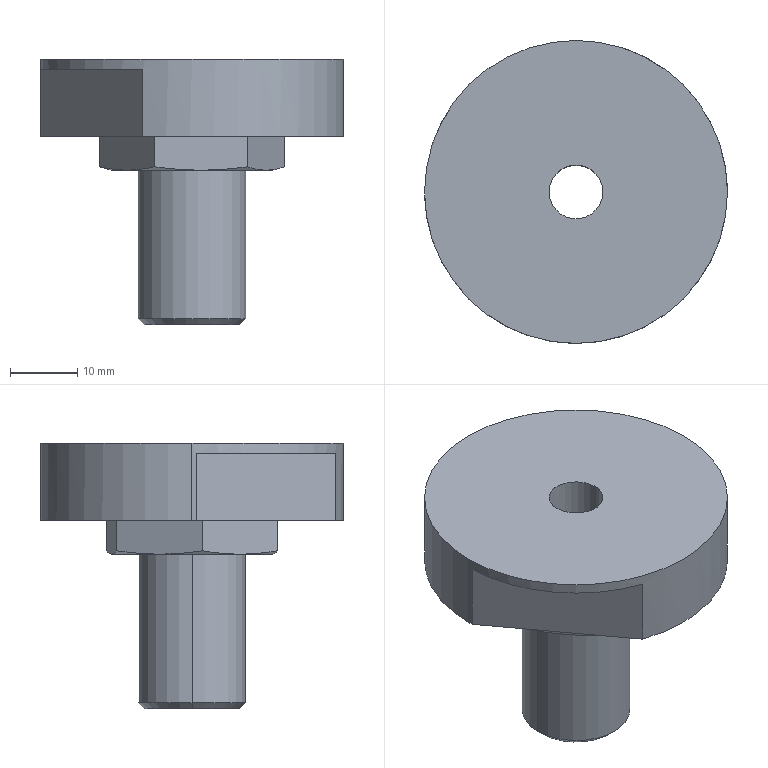Part | SolidWorks | features BaseBody 1 | 1 solid | 34 faces | box 45 x 45 x 39.5 mm | volume 21967 mm3 | plane 14 | cone 12 | cylinder 8 | commonest cylinder face diameters 8 x2 8.566 x2 16 x2 45 x2
STEP:
#1=CARTESIAN_POINT('',(67.28,21.29,385.481));
#2=VERTEX_POINT('',#1);
#3=CARTESIAN_POINT('',(37.5,0.,385.481));
#4=VERTEX_POINT('',#3);
#5=CARTESIAN_POINT('',(60.,0.,385.481));
#6=DIRECTION('',(0.,0.,1.));
#7=DIRECTION('',(1.,0.,0.));
#8=AXIS2_PLACEMENT_3D('',#5,#6,#7);
#9=CIRCLE('',#8,22.5);
#10=EDGE_CURVE('',#2,#4,#9,.T.);
#11=ORIENTED_EDGE('',*,*,#10,.T.);
#12=CARTESIAN_POINT('',(37.5,0.,396.981));
#13=VERTEX_POINT('',#12);
#14=CARTESIAN_POINT('',(37.5,0.,391.231));
#15=DIRECTION('',(0.,0.,1.));
#16=VECTOR('',#15,1000.);
#17=LINE('',#14,#16);
#18=EDGE_CURVE('',#4,#13,#17,.T.);
#19=ORIENTED_EDGE('',*,*,#18,.T.);
#20=CARTESIAN_POINT('',(82.5,0.,396.981));
#21=VERTEX_POINT('',#20);
#22=CARTESIAN_POINT('',(60.,0.,396.981));
#23=DIRECTION('',(0.,0.,1.));
#24=DIRECTION('',(1.,0.,0.));
#25=AXIS2_PLACEMENT_3D('',#22,#23,#24);
#26=CIRCLE('',#25,22.5);
#27=EDGE_CURVE('',#21,#13,#26,.T.);
#28=ORIENTED_EDGE('',*,*,#27,.F.);
#29=CARTESIAN_POINT('',(82.5,0.,385.481));
#30=VERTEX_POINT('',#29);
#31=CARTESIAN_POINT('',(82.5,0.,391.231));
#32=DIRECTION('',(0.,0.,1.));
#33=VECTOR('',#32,1000.);
#34=LINE('',#31,#33);
#35=EDGE_CURVE('',#30,#21,#34,.T.);
#36=ORIENTED_EDGE('',*,*,#35,.F.);
#37=CARTESIAN_POINT('',(82.49,0.6822,385.481));
#38=VERTEX_POINT('',#37);
#39=CARTESIAN_POINT('',(60.,0.,385.481));
#40=DIRECTION('',(0.,0.,1.));
#41=DIRECTION('',(1.,0.,0.));
#42=AXIS2_PLACEMENT_3D('',#39,#40,#41);
#43=CIRCLE('',#42,22.5);
#44=EDGE_CURVE('',#30,#38,#43,.T.);
#45=ORIENTED_EDGE('',*,*,#44,.T.);
#46=CARTESIAN_POINT('',(82.49,0.6822,395.481));
#47=VERTEX_POINT('',#46);
#48=CARTESIAN_POINT('',(82.49,0.6822,391.231));
#49=DIRECTION('',(0.,0.,1.));
#50=VECTOR('',#49,1000.);
#51=LINE('',#48,#50);
#52=EDGE_CURVE('',#38,#47,#51,.T.);
#53=ORIENTED_EDGE('',*,*,#52,.T.);
#54=CARTESIAN_POINT('',(67.28,21.29,395.481));
#55=VERTEX_POINT('',#54);
#56=CARTESIAN_POINT('',(60.,0.,395.481));
#57=DIRECTION('',(0.,0.,1.));
#58=DIRECTION('',(1.,0.,0.));
#59=AXIS2_PLACEMENT_3D('',#56,#57,#58);
#60=CIRCLE('',#59,22.5);
#61=EDGE_CURVE('',#47,#55,#60,.T.);
#62=ORIENTED_EDGE('',*,*,#61,.T.);
#63=CARTESIAN_POINT('',(67.28,21.29,391.231));
#64=DIRECTION('',(0.,0.,-1.));
#65=VECTOR('',#64,1000.);
#66=LINE('',#63,#65);
#67=EDGE_CURVE('',#55,#2,#66,.T.);
#68=ORIENTED_EDGE('',*,*,#67,.T.);
#69=EDGE_LOOP('',(#11,#19,#28,#36,#45,#53,#62,#68));
#70=FACE_OUTER_BOUND('',#69,.T.);
#71=CARTESIAN_POINT('',(60.,0.,391.231));
#72=DIRECTION('',(0.,0.,1.));
#73=DIRECTION('',(1.,0.,0.));
#74=AXIS2_PLACEMENT_3D('',#71,#72,#73);
#75=CYLINDRICAL_SURFACE('',#74,22.5);
#76=ADVANCED_FACE('',(#70),#75,.T.);
#77=CARTESIAN_POINT('',(56.,0.,361.844));
#78=VERTEX_POINT('',#77);
#79=CARTESIAN_POINT('',(64.,0.,361.844));
#80=VERTEX_POINT('',#79);
#81=CARTESIAN_POINT('',(60.,0.,361.844));
#82=DIRECTION('',(0.,0.,1.));
#83=DIRECTION('',(1.,0.,0.));
#84=AXIS2_PLACEMENT_3D('',#81,#82,#83);
#85=CIRCLE('',#84,4.);
#86=EDGE_CURVE('',#78,#80,#85,.T.);
#87=ORIENTED_EDGE('',*,*,#86,.F.);
#88=CARTESIAN_POINT('',(56.,0.,396.981));
#89=VERTEX_POINT('',#88);
#90=CARTESIAN_POINT('',(56.,0.,379.413));
#91=DIRECTION('',(0.,0.,1.));
#92=VECTOR('',#91,1000.);
#93=LINE('',#90,#92);
#94=EDGE_CURVE('',#78,#89,#93,.T.);
#95=ORIENTED_EDGE('',*,*,#94,.T.);
#96=CARTESIAN_POINT('',(64.,0.,396.981));
#97=VERTEX_POINT('',#96);
#98=CARTESIAN_POINT('',(60.,0.,396.981));
#99=DIRECTION('',(0.,0.,-1.));
#100=DIRECTION('',(1.,0.,0.));
#101=AXIS2_PLACEMENT_3D('',#98,#99,#100);
#102=CIRCLE('',#101,4.);
#103=EDGE_CURVE('',#97,#89,#102,.T.);
#104=ORIENTED_EDGE('',*,*,#103,.F.);
#105=CARTESIAN_POINT('',(64.,0.,379.413));
#106=DIRECTION('',(0.,0.,1.));
#107=VECTOR('',#106,1000.);
#108=LINE('',#105,#107);
#109=EDGE_CURVE('',#80,#97,#108,.T.);
#110=ORIENTED_EDGE('',*,*,#109,.F.);
#111=EDGE_LOOP('',(#87,#95,#104,#110));
#112=FACE_OUTER_BOUND('',#111,.T.);
#113=CARTESIAN_POINT('',(60.,0.,379.413));
#114=DIRECTION('',(0.,0.,1.));
#115=DIRECTION('',(1.,0.,0.));
#116=AXIS2_PLACEMENT_3D('',#113,#114,#115);
#117=CYLINDRICAL_SURFACE('',#116,4.);
#118=ADVANCED_FACE('',(#112),#117,.F.);
#119=ORIENTED_EDGE('',*,*,#86,.T.);
#120=CARTESIAN_POINT('',(64.283,0.,361.681));
#121=VERTEX_POINT('',#120);
#122=CARTESIAN_POINT('',(64.283,0.,361.681));
#123=DIRECTION('',(0.866,0.,-0.5));
#124=VECTOR('',#123,1000.);
#125=LINE('',#122,#124);
#126=EDGE_CURVE('',#80,#121,#125,.T.);
#127=ORIENTED_EDGE('',*,*,#126,.T.);
#128=CARTESIAN_POINT('',(55.717,0.,361.681));
#129=VERTEX_POINT('',#128);
#130=CARTESIAN_POINT('',(60.,0.,361.681));
#131=DIRECTION('',(0.,0.,1.));
#132=DIRECTION('',(-0.8046,-0.5938,0.));
#133=AXIS2_PLACEMENT_3D('',#130,#131,#132);
#134=CIRCLE('',#133,4.283);
#135=EDGE_CURVE('',#129,#121,#134,.T.);
#136=ORIENTED_EDGE('',*,*,#135,.F.);
#137=CARTESIAN_POINT('',(55.717,0.,361.681));
#138=DIRECTION('',(-0.866,0.,-0.5));
#139=VECTOR('',#138,1000.);
#140=LINE('',#137,#139);
#141=EDGE_CURVE('',#78,#129,#140,.T.);
#142=ORIENTED_EDGE('',*,*,#141,.F.);
#143=EDGE_LOOP('',(#119,#127,#136,#142));
#144=FACE_OUTER_BOUND('',#143,.T.);
#145=CARTESIAN_POINT('',(60.,0.,361.681));
#146=DIRECTION('',(0.,0.,-1.));
#147=DIRECTION('',(-1.,0.,0.));
#148=AXIS2_PLACEMENT_3D('',#145,#146,#147);
#149=CONICAL_SURFACE('',#148,4.283,1.047);
#150=ADVANCED_FACE('',(#144),#149,.F.);
#151=CARTESIAN_POINT('',(55.717,0.,358.062));
#152=VERTEX_POINT('',#151);
#153=CARTESIAN_POINT('',(64.283,0.,358.062));
#154=VERTEX_POINT('',#153);
#155=CARTESIAN_POINT('',(60.,0.,358.062));
#156=DIRECTION('',(0.,0.,1.));
#157=DIRECTION('',(1.,0.,0.));
#158=AXIS2_PLACEMENT_3D('',#155,#156,#157);
#159=CIRCLE('',#158,4.283);
#160=EDGE_CURVE('',#152,#154,#159,.T.);
#161=ORIENTED_EDGE('',*,*,#160,.F.);
#162=CARTESIAN_POINT('',(55.717,0.,358.872));
#163=DIRECTION('',(0.,0.,1.));
#164=VECTOR('',#163,1000.);
#165=LINE('',#162,#164);
#166=EDGE_CURVE('',#152,#129,#165,.T.);
#167=ORIENTED_EDGE('',*,*,#166,.T.);
#168=ORIENTED_EDGE('',*,*,#135,.T.);
#169=CARTESIAN_POINT('',(64.283,0.,358.872));
#170=DIRECTION('',(0.,0.,1.));
#171=VECTOR('',#170,1000.);
#172=LINE('',#169,#171);
#173=EDGE_CURVE('',#154,#121,#172,.T.);
#174=ORIENTED_EDGE('',*,*,#173,.F.);
#175=EDGE_LOOP('',(#161,#167,#168,#174));
#176=FACE_OUTER_BOUND('',#175,.T.);
#177=CARTESIAN_POINT('',(60.,0.,358.872));
#178=DIRECTION('',(0.,0.,1.));
#179=DIRECTION('',(1.,0.,0.));
#180=AXIS2_PLACEMENT_3D('',#177,#178,#179);
#181=CYLINDRICAL_SURFACE('',#180,4.283);
#182=ADVANCED_FACE('',(#176),#181,.F.);
#183=ORIENTED_EDGE('',*,*,#160,.T.);
#184=CARTESIAN_POINT('',(64.864,0.,357.481));
#185=VERTEX_POINT('',#184);
#186=CARTESIAN_POINT('',(64.864,0.,357.481));
#187=DIRECTION('',(0.7071,0.,-0.7071));
#188=VECTOR('',#187,1000.);
#189=LINE('',#186,#188);
#190=EDGE_CURVE('',#154,#185,#189,.T.);
#191=ORIENTED_EDGE('',*,*,#190,.T.);
#192=CARTESIAN_POINT('',(55.136,0.,357.481));
#193=VERTEX_POINT('',#192);
#194=CARTESIAN_POINT('',(60.,0.,357.481));
#195=DIRECTION('',(0.,0.,1.));
#196=DIRECTION('',(-1.,0.,0.));
#197=AXIS2_PLACEMENT_3D('',#194,#195,#196);
#198=CIRCLE('',#197,4.864);
#199=EDGE_CURVE('',#193,#185,#198,.T.);
#200=ORIENTED_EDGE('',*,*,#199,.F.);
#201=CARTESIAN_POINT('',(55.136,0.,357.481));
#202=DIRECTION('',(-0.7071,0.,-0.7071));
#203=VECTOR('',#202,1000.);
#204=LINE('',#201,#203);
#205=EDGE_CURVE('',#152,#193,#204,.T.);
#206=ORIENTED_EDGE('',*,*,#205,.F.);
#207=EDGE_LOOP('',(#183,#191,#200,#206));
#208=FACE_OUTER_BOUND('',#207,.T.);
#209=CARTESIAN_POINT('',(60.,0.,357.481));
#210=DIRECTION('',(0.,0.,-1.));
#211=DIRECTION('',(-1.,0.,0.));
#212=AXIS2_PLACEMENT_3D('',#209,#210,#211);
#213=CONICAL_SURFACE('',#212,4.864,0.7854);
#214=ADVANCED_FACE('',(#208),#213,.F.);
#215=CARTESIAN_POINT('',(68.,0.,358.401));
#216=VERTEX_POINT('',#215);
#217=CARTESIAN_POINT('',(52.,0.,358.401));
#218=VERTEX_POINT('',#217);
#219=CARTESIAN_POINT('',(60.,0.,358.401));
#220=DIRECTION('',(0.,0.,1.));
#221=DIRECTION('',(1.,0.,0.));
#222=AXIS2_PLACEMENT_3D('',#219,#220,#221);
#223=CIRCLE('',#222,8.);
#224=EDGE_CURVE('',#216,#218,#223,.T.);
#225=ORIENTED_EDGE('',*,*,#224,.T.);
#226=CARTESIAN_POINT('',(52.,0.,380.481));
#227=VERTEX_POINT('',#226);
#228=CARTESIAN_POINT('',(52.,0.,368.441));
#229=DIRECTION('',(0.,0.,1.));
#230=VECTOR('',#229,1000.);
#231=LINE('',#228,#230);
#232=EDGE_CURVE('',#218,#227,#231,.T.);
#233=ORIENTED_EDGE('',*,*,#232,.T.);
#234=CARTESIAN_POINT('',(68.,0.,380.481));
#235=VERTEX_POINT('',#234);
#236=CARTESIAN_POINT('',(60.,0.,380.481));
#237=DIRECTION('',(0.,0.,1.));
#238=DIRECTION('',(1.,0.,0.));
#239=AXIS2_PLACEMENT_3D('',#236,#237,#238);
#240=CIRCLE('',#239,8.);
#241=EDGE_CURVE('',#235,#227,#240,.T.);
#242=ORIENTED_EDGE('',*,*,#241,.F.);
#243=CARTESIAN_POINT('',(68.,0.,368.441));
#244=DIRECTION('',(0.,0.,1.));
#245=VECTOR('',#244,1000.);
#246=LINE('',#243,#245);
#247=EDGE_CURVE('',#216,#235,#246,.T.);
#248=ORIENTED_EDGE('',*,*,#247,.F.);
#249=EDGE_LOOP('',(#225,#233,#242,#248));
#250=FACE_OUTER_BOUND('',#249,.T.);
#251=CARTESIAN_POINT('',(60.,0.,368.441));
#252=DIRECTION('',(0.,0.,1.));
#253=DIRECTION('',(1.,0.,0.));
#254=AXIS2_PLACEMENT_3D('',#251,#252,#253);
#255=CYLINDRICAL_SURFACE('',#254,8.);
#256=ADVANCED_FACE('',(#250),#255,.T.);
#257=CARTESIAN_POINT('',(52.92,0.,357.481));
#258=VERTEX_POINT('',#257);
#259=CARTESIAN_POINT('',(67.08,0.,357.481));
#260=VERTEX_POINT('',#259);
#261=CARTESIAN_POINT('',(60.,0.,357.481));
#262=DIRECTION('',(0.,0.,-1.));
#263=DIRECTION('',(1.,0.,0.));
#264=AXIS2_PLACEMENT_3D('',#261,#262,#263);
#265=CIRCLE('',#264,7.08);
#266=EDGE_CURVE('',#258,#260,#265,.T.);
#267=ORIENTED_EDGE('',*,*,#266,.F.);
#268=CARTESIAN_POINT('',(52.,0.,358.401));
#269=DIRECTION('',(-0.7071,0.,0.7071));
#270=VECTOR('',#269,1000.);
#271=LINE('',#268,#270);
#272=EDGE_CURVE('',#258,#218,#271,.T.);
#273=ORIENTED_EDGE('',*,*,#272,.T.);
#274=ORIENTED_EDGE('',*,*,#224,.F.);
#275=CARTESIAN_POINT('',(68.,0.,358.401));
#276=DIRECTION('',(0.7071,0.,0.7071));
#277=VECTOR('',#276,1000.);
#278=LINE('',#275,#277);
#279=EDGE_CURVE('',#260,#216,#278,.T.);
#280=ORIENTED_EDGE('',*,*,#279,.F.);
#281=EDGE_LOOP('',(#267,#273,#274,#280));
#282=FACE_OUTER_BOUND('',#281,.T.);
#283=CARTESIAN_POINT('',(60.,0.,358.401));
#284=DIRECTION('',(0.,0.,1.));
#285=DIRECTION('',(1.,0.,0.));
#286=AXIS2_PLACEMENT_3D('',#283,#284,#285);
#287=CONICAL_SURFACE('',#286,8.,0.7854);
#288=ADVANCED_FACE('',(#282),#287,.T.);
#289=ORIENTED_EDGE('',*,*,#27,.T.);
#290=CARTESIAN_POINT('',(60.,0.,396.981));
#291=DIRECTION('',(0.,0.,1.));
#292=DIRECTION('',(1.,0.,0.));
#293=AXIS2_PLACEMENT_3D('',#290,#291,#292);
#294=CIRCLE('',#293,22.5);
#295=EDGE_CURVE('',#13,#21,#294,.T.);
#296=ORIENTED_EDGE('',*,*,#295,.T.);
#297=EDGE_LOOP('',(#289,#296));
#298=FACE_OUTER_BOUND('',#297,.T.);
#299=ORIENTED_EDGE('',*,*,#103,.T.);
#300=CARTESIAN_POINT('',(60.,0.,396.981));
#301=DIRECTION('',(0.,0.,-1.));
#302=DIRECTION('',(1.,0.,0.));
#303=AXIS2_PLACEMENT_3D('',#300,#301,#302);
#304=CIRCLE('',#303,4.);
#305=EDGE_CURVE('',#89,#97,#304,.T.);
#306=ORIENTED_EDGE('',*,*,#305,.T.);
#307=EDGE_LOOP('',(#299,#306));
#308=FACE_BOUND('',#307,.T.);
#309=CARTESIAN_POINT('',(52.132,10.661,396.981));
#310=DIRECTION('',(0.,0.,1.));
#311=DIRECTION('',(1.,0.,0.));
#312=AXIS2_PLACEMENT_3D('',#309,#310,#311);
#313=PLANE('',#312);
#314=ADVANCED_FACE('',(#298,#308),#313,.T.);
#315=ORIENTED_EDGE('',*,*,#18,.F.);
#316=CARTESIAN_POINT('',(37.51,-0.6822,385.481));
#317=VERTEX_POINT('',#316);
#318=CARTESIAN_POINT('',(60.,0.,385.481));
#319=DIRECTION('',(0.,0.,1.));
#320=DIRECTION('',(1.,0.,0.));
#321=AXIS2_PLACEMENT_3D('',#318,#319,#320);
#322=CIRCLE('',#321,22.5);
#323=EDGE_CURVE('',#4,#317,#322,.T.);
#324=ORIENTED_EDGE('',*,*,#323,.T.);
#325=CARTESIAN_POINT('',(37.51,-0.6822,395.481));
#326=VERTEX_POINT('',#325);
#327=CARTESIAN_POINT('',(37.51,-0.6822,391.231));
#328=DIRECTION('',(0.,0.,1.));
#329=VECTOR('',#328,1000.);
#330=LINE('',#327,#329);
#331=EDGE_CURVE('',#317,#326,#330,.T.);
#332=ORIENTED_EDGE('',*,*,#331,.T.);
#333=CARTESIAN_POINT('',(52.72,-21.29,395.481));
#334=VERTEX_POINT('',#333);
#335=CARTESIAN_POINT('',(60.,0.,395.481));
#336=DIRECTION('',(0.,0.,1.));
#337=DIRECTION('',(1.,0.,0.));
#338=AXIS2_PLACEMENT_3D('',#335,#336,#337);
#339=CIRCLE('',#338,22.5);
#340=EDGE_CURVE('',#326,#334,#339,.T.);
#341=ORIENTED_EDGE('',*,*,#340,.T.);
#342=CARTESIAN_POINT('',(52.72,-21.29,385.481));
#343=VERTEX_POINT('',#342);
#344=CARTESIAN_POINT('',(52.72,-21.29,391.231));
#345=DIRECTION('',(0.,0.,-1.));
#346=VECTOR('',#345,1000.);
#347=LINE('',#344,#346);
#348=EDGE_CURVE('',#334,#343,#347,.T.);
#349=ORIENTED_EDGE('',*,*,#348,.T.);
#350=CARTESIAN_POINT('',(60.,0.,385.481));
#351=DIRECTION('',(0.,0.,1.));
#352=DIRECTION('',(1.,0.,0.));
#353=AXIS2_PLACEMENT_3D('',#350,#351,#352);
#354=CIRCLE('',#353,22.5);
#355=EDGE_CURVE('',#343,#30,#354,.T.);
#356=ORIENTED_EDGE('',*,*,#355,.T.);
#357=ORIENTED_EDGE('',*,*,#35,.T.);
#358=ORIENTED_EDGE('',*,*,#295,.F.);
#359=EDGE_LOOP('',(#315,#324,#332,#341,#349,#356,#357,#358));
#360=FACE_OUTER_BOUND('',#359,.T.);
#361=CARTESIAN_POINT('',(60.,0.,391.231));
#362=DIRECTION('',(0.,0.,1.));
#363=DIRECTION('',(1.,0.,0.));
#364=AXIS2_PLACEMENT_3D('',#361,#362,#363);
#365=CYLINDRICAL_SURFACE('',#364,22.5);
#366=ADVANCED_FACE('',(#360),#365,.T.);
#367=ORIENTED_EDGE('',*,*,#94,.F.);
#368=CARTESIAN_POINT('',(60.,0.,361.844));
#369=DIRECTION('',(0.,0.,1.));
#370=DIRECTION('',(1.,0.,0.));
#371=AXIS2_PLACEMENT_3D('',#368,#369,#370);
#372=CIRCLE('',#371,4.);
#373=EDGE_CURVE('',#80,#78,#372,.T.);
#374=ORIENTED_EDGE('',*,*,#373,.F.);
#375=ORIENTED_EDGE('',*,*,#109,.T.);
#376=ORIENTED_EDGE('',*,*,#305,.F.);
#377=EDGE_LOOP('',(#367,#374,#375,#376));
#378=FACE_OUTER_BOUND('',#377,.T.);
#379=CARTESIAN_POINT('',(60.,0.,379.413));
#380=DIRECTION('',(0.,0.,1.));
#381=DIRECTION('',(1.,0.,0.));
#382=AXIS2_PLACEMENT_3D('',#379,#380,#381);
#383=CYLINDRICAL_SURFACE('',#382,4.);
#384=ADVANCED_FACE('',(#378),#383,.F.);
#385=CARTESIAN_POINT('',(52.72,-21.29,385.481));
#386=DIRECTION('',(-0.5938,0.8046,0.));
#387=VECTOR('',#386,1000.);
#388=LINE('',#385,#387);
#389=EDGE_CURVE('',#343,#317,#388,.T.);
#390=ORIENTED_EDGE('',*,*,#389,.T.);
#391=ORIENTED_EDGE('',*,*,#323,.F.);
#392=ORIENTED_EDGE('',*,*,#10,.F.);
#393=CARTESIAN_POINT('',(67.28,21.29,385.481));
#394=DIRECTION('',(0.5938,-0.8046,0.));
#395=VECTOR('',#394,1000.);
#396=LINE('',#393,#395);
#397=EDGE_CURVE('',#2,#38,#396,.T.);
#398=ORIENTED_EDGE('',*,*,#397,.T.);
#399=ORIENTED_EDGE('',*,*,#44,.F.);
#400=ORIENTED_EDGE('',*,*,#355,.F.);
#401=EDGE_LOOP('',(#390,#391,#392,#398,#399,#400));
#402=FACE_OUTER_BOUND('',#401,.T.);
#403=CARTESIAN_POINT('',(65.541,12.7,385.481));
#404=VERTEX_POINT('',#403);
#405=CARTESIAN_POINT('',(51.772,11.149,385.481));
#406=VERTEX_POINT('',#405);
#407=CARTESIAN_POINT('',(65.541,12.7,385.481));
#408=DIRECTION('',(-0.9937,-0.112,0.));
#409=VECTOR('',#408,1000.);
#410=LINE('',#407,#409);
#411=EDGE_CURVE('',#404,#406,#410,.T.);
#412=ORIENTED_EDGE('',*,*,#411,.T.);
#413=CARTESIAN_POINT('',(46.231,-1.552,385.481));
#414=VERTEX_POINT('',#413);
#415=CARTESIAN_POINT('',(51.772,11.149,385.481));
#416=DIRECTION('',(-0.3999,-0.9166,0.));
#417=VECTOR('',#416,1000.);
#418=LINE('',#415,#417);
#419=EDGE_CURVE('',#406,#414,#418,.T.);
#420=ORIENTED_EDGE('',*,*,#419,.T.);
#421=CARTESIAN_POINT('',(54.459,-12.7,385.481));
#422=VERTEX_POINT('',#421);
#423=CARTESIAN_POINT('',(46.231,-1.552,385.481));
#424=DIRECTION('',(0.5938,-0.8046,0.));
#425=VECTOR('',#424,1000.);
#426=LINE('',#423,#425);
#427=EDGE_CURVE('',#414,#422,#426,.T.);
#428=ORIENTED_EDGE('',*,*,#427,.T.);
#429=CARTESIAN_POINT('',(68.228,-11.149,385.481));
#430=VERTEX_POINT('',#429);
#431=CARTESIAN_POINT('',(54.459,-12.7,385.481));
#432=DIRECTION('',(0.9937,0.112,0.));
#433=VECTOR('',#432,1000.);
#434=LINE('',#431,#433);
#435=EDGE_CURVE('',#422,#430,#434,.T.);
#436=ORIENTED_EDGE('',*,*,#435,.T.);
#437=CARTESIAN_POINT('',(73.769,1.552,385.481));
#438=VERTEX_POINT('',#437);
#439=CARTESIAN_POINT('',(68.228,-11.149,385.481));
#440=DIRECTION('',(0.3999,0.9166,0.));
#441=VECTOR('',#440,1000.);
#442=LINE('',#439,#441);
#443=EDGE_CURVE('',#430,#438,#442,.T.);
#444=ORIENTED_EDGE('',*,*,#443,.T.);
#445=CARTESIAN_POINT('',(73.769,1.552,385.481));
#446=DIRECTION('',(-0.5938,0.8046,0.));
#447=VECTOR('',#446,1000.);
#448=LINE('',#445,#447);
#449=EDGE_CURVE('',#438,#404,#448,.T.);
#450=ORIENTED_EDGE('',*,*,#449,.T.);
#451=EDGE_LOOP('',(#412,#420,#428,#436,#444,#450));
#452=FACE_BOUND('',#451,.T.);
#453=CARTESIAN_POINT('',(47.619,16.776,385.481));
#454=DIRECTION('',(0.,0.,-1.));
#455=DIRECTION('',(-1.,0.,0.));
#456=AXIS2_PLACEMENT_3D('',#453,#454,#455);
#457=PLANE('',#456);
#458=ADVANCED_FACE('',(#402,#452),#457,.T.);
#459=ORIENTED_EDGE('',*,*,#67,.F.);
#460=CARTESIAN_POINT('',(51.131,43.169,395.481));
#461=DIRECTION('',(-0.5938,0.8046,0.));
#462=VECTOR('',#461,1000.);
#463=LINE('',#460,#462);
#464=EDGE_CURVE('',#47,#55,#463,.T.);
#465=ORIENTED_EDGE('',*,*,#464,.F.);
#466=ORIENTED_EDGE('',*,*,#52,.F.);
#467=ORIENTED_EDGE('',*,*,#397,.F.);
#468=EDGE_LOOP('',(#459,#465,#466,#467));
#469=FACE_OUTER_BOUND('',#468,.T.);
#470=CARTESIAN_POINT('',(51.131,43.169,395.481));
#471=DIRECTION('',(-0.8046,-0.5938,0.));
#472=DIRECTION('',(0.5938,-0.8046,0.));
#473=AXIS2_PLACEMENT_3D('',#470,#471,#472);
#474=PLANE('',#473);
#475=ADVANCED_FACE('',(#469),#474,.F.);
#476=ORIENTED_EDGE('',*,*,#61,.F.);
#477=ORIENTED_EDGE('',*,*,#464,.T.);
#478=EDGE_LOOP('',(#476,#477));
#479=FACE_OUTER_BOUND('',#478,.T.);
#480=CARTESIAN_POINT('',(60.,0.,395.481));
#481=DIRECTION('',(0.,0.,-1.));
#482=DIRECTION('',(-1.,0.,0.));
#483=AXIS2_PLACEMENT_3D('',#480,#481,#482);
#484=PLANE('',#483);
#485=ADVANCED_FACE('',(#479),#484,.T.);
#486=ORIENTED_EDGE('',*,*,#348,.F.);
#487=CARTESIAN_POINT('',(68.869,-43.169,395.481));
#488=DIRECTION('',(0.5938,-0.8046,0.));
#489=VECTOR('',#488,1000.);
#490=LINE('',#487,#489);
#491=EDGE_CURVE('',#326,#334,#490,.T.);
#492=ORIENTED_EDGE('',*,*,#491,.F.);
#493=ORIENTED_EDGE('',*,*,#331,.F.);
#494=ORIENTED_EDGE('',*,*,#389,.F.);
#495=EDGE_LOOP('',(#486,#492,#493,#494));
#496=FACE_OUTER_BOUND('',#495,.T.);
#497=CARTESIAN_POINT('',(68.869,-43.169,395.481));
#498=DIRECTION('',(0.8046,0.5938,0.));
#499=DIRECTION('',(-0.5938,0.8046,0.));
#500=AXIS2_PLACEMENT_3D('',#497,#498,#499);
#501=PLANE('',#500);
#502=ADVANCED_FACE('',(#496),#501,.F.);
#503=ORIENTED_EDGE('',*,*,#340,.F.);
#504=ORIENTED_EDGE('',*,*,#491,.T.);
#505=EDGE_LOOP('',(#503,#504));
#506=FACE_OUTER_BOUND('',#505,.T.);
#507=CARTESIAN_POINT('',(60.,0.,395.481));
#508=DIRECTION('',(0.,0.,-1.));
#509=DIRECTION('',(-1.,0.,0.));
#510=AXIS2_PLACEMENT_3D('',#507,#508,#509);
#511=PLANE('',#510);
#512=ADVANCED_FACE('',(#506),#511,.T.);
#513=ORIENTED_EDGE('',*,*,#126,.F.);
#514=ORIENTED_EDGE('',*,*,#373,.T.);
#515=ORIENTED_EDGE('',*,*,#141,.T.);
#516=CARTESIAN_POINT('',(60.,0.,361.681));
#517=DIRECTION('',(0.,0.,1.));
#518=DIRECTION('',(-0.8046,-0.5938,0.));
#519=AXIS2_PLACEMENT_3D('',#516,#517,#518);
#520=CIRCLE('',#519,4.283);
#521=EDGE_CURVE('',#121,#129,#520,.T.);
#522=ORIENTED_EDGE('',*,*,#521,.F.);
#523=EDGE_LOOP('',(#513,#514,#515,#522));
#524=FACE_OUTER_BOUND('',#523,.T.);
#525=CARTESIAN_POINT('',(60.,0.,361.681));
#526=DIRECTION('',(0.,0.,-1.));
#527=DIRECTION('',(-1.,0.,0.));
#528=AXIS2_PLACEMENT_3D('',#525,#526,#527);
#529=CONICAL_SURFACE('',#528,4.283,1.047);
#530=ADVANCED_FACE('',(#524),#529,.F.);
#531=CARTESIAN_POINT('',(46.231,-1.552,380.978));
#532=VERTEX_POINT('',#531);
#533=CARTESIAN_POINT('',(46.231,-1.552,385.481));
#534=DIRECTION('',(0.,0.,-1.));
#535=VECTOR('',#534,1000.);
#536=LINE('',#533,#535);
#537=EDGE_CURVE('',#414,#532,#536,.T.);
#538=ORIENTED_EDGE('',*,*,#537,.F.);
#539=ORIENTED_EDGE('',*,*,#419,.F.);
#540=CARTESIAN_POINT('',(51.772,11.149,380.978));
#541=VERTEX_POINT('',#540);
#542=CARTESIAN_POINT('',(51.772,11.149,385.481));
#543=DIRECTION('',(0.,0.,1.));
#544=VECTOR('',#543,1000.);
#545=LINE('',#542,#544);
#546=EDGE_CURVE('',#541,#406,#545,.T.);
#547=ORIENTED_EDGE('',*,*,#546,.F.);
#548=CARTESIAN_POINT('',(49.001,4.798,380.481));
#549=VERTEX_POINT('',#548);
#550=CARTESIAN_POINT('',(49.001,4.798,380.481));
#551=CARTESIAN_POINT('',(49.465,5.862,380.481));
#552=CARTESIAN_POINT('',(49.928,6.923,380.527));
#553=CARTESIAN_POINT('',(50.851,9.039,380.699));
#554=CARTESIAN_POINT('',(51.312,10.095,380.824));
#555=CARTESIAN_POINT('',(51.772,11.149,380.978));
#556=B_SPLINE_CURVE_WITH_KNOTS('',3,(#550,#551,#552,#553,#554,#555),.UNSPECIFIED.,.F.,.F.,(4,2,4),(0.,0.003473,0.006946),.UNSPECIFIED.);
#557=EDGE_CURVE('',#549,#541,#556,.T.);
#558=ORIENTED_EDGE('',*,*,#557,.F.);
#559=CARTESIAN_POINT('',(46.231,-1.552,380.978));
#560=CARTESIAN_POINT('',(46.69,-0.498,380.824));
#561=CARTESIAN_POINT('',(47.151,0.5576,380.699));
#562=CARTESIAN_POINT('',(48.074,2.674,380.527));
#563=CARTESIAN_POINT('',(48.537,3.735,380.481));
#564=CARTESIAN_POINT('',(49.001,4.798,380.481));
#565=B_SPLINE_CURVE_WITH_KNOTS('',3,(#559,#560,#561,#562,#563,#564),.UNSPECIFIED.,.F.,.F.,(4,2,4),(0.,0.003473,0.006946),.UNSPECIFIED.);
#566=EDGE_CURVE('',#532,#549,#565,.T.);
#567=ORIENTED_EDGE('',*,*,#566,.F.);
#568=EDGE_LOOP('',(#538,#539,#547,#558,#567));
#569=FACE_OUTER_BOUND('',#568,.T.);
#570=CARTESIAN_POINT('',(46.231,-1.552,385.481));
#571=DIRECTION('',(0.9166,-0.3999,0.));
#572=DIRECTION('',(0.3999,0.9166,0.));
#573=AXIS2_PLACEMENT_3D('',#570,#571,#572);
#574=PLANE('',#573);
#575=ADVANCED_FACE('',(#569),#574,.F.);
#576=ORIENTED_EDGE('',*,*,#411,.F.);
#577=CARTESIAN_POINT('',(65.541,12.7,380.978));
#578=VERTEX_POINT('',#577);
#579=CARTESIAN_POINT('',(65.541,12.7,385.481));
#580=DIRECTION('',(0.,0.,1.));
#581=VECTOR('',#580,1000.);
#582=LINE('',#579,#581);
#583=EDGE_CURVE('',#578,#404,#582,.T.);
#584=ORIENTED_EDGE('',*,*,#583,.F.);
#585=CARTESIAN_POINT('',(58.656,11.925,380.481));
#586=VERTEX_POINT('',#585);
#587=CARTESIAN_POINT('',(58.656,11.925,380.481));
#588=CARTESIAN_POINT('',(59.81,12.054,380.481));
#589=CARTESIAN_POINT('',(60.96,12.184,380.527));
#590=CARTESIAN_POINT('',(63.254,12.443,380.699));
#591=CARTESIAN_POINT('',(64.398,12.572,380.824));
#592=CARTESIAN_POINT('',(65.541,12.7,380.978));
#593=B_SPLINE_CURVE_WITH_KNOTS('',3,(#587,#588,#589,#590,#591,#592),.UNSPECIFIED.,.F.,.F.,(4,2,4),(0.,0.003473,0.006946),.UNSPECIFIED.);
#594=EDGE_CURVE('',#586,#578,#593,.T.);
#595=ORIENTED_EDGE('',*,*,#594,.F.);
#596=CARTESIAN_POINT('',(51.772,11.149,380.978));
#597=CARTESIAN_POINT('',(52.914,11.277,380.824));
#598=CARTESIAN_POINT('',(54.058,11.406,380.699));
#599=CARTESIAN_POINT('',(56.353,11.665,380.527));
#600=CARTESIAN_POINT('',(57.503,11.795,380.481));
#601=CARTESIAN_POINT('',(58.656,11.925,380.481));
#602=B_SPLINE_CURVE_WITH_KNOTS('',3,(#596,#597,#598,#599,#600,#601),.UNSPECIFIED.,.F.,.F.,(4,2,4),(0.,0.003473,0.006946),.UNSPECIFIED.);
#603=EDGE_CURVE('',#541,#586,#602,.T.);
#604=ORIENTED_EDGE('',*,*,#603,.F.);
#605=ORIENTED_EDGE('',*,*,#546,.T.);
#606=EDGE_LOOP('',(#576,#584,#595,#604,#605));
#607=FACE_OUTER_BOUND('',#606,.T.);
#608=CARTESIAN_POINT('',(51.772,11.149,385.481));
#609=DIRECTION('',(0.112,-0.9937,0.));
#610=DIRECTION('',(0.9937,0.112,0.));
#611=AXIS2_PLACEMENT_3D('',#608,#609,#610);
#612=PLANE('',#611);
#613=ADVANCED_FACE('',(#607),#612,.F.);
#614=ORIENTED_EDGE('',*,*,#449,.F.);
#615=CARTESIAN_POINT('',(73.769,1.552,380.978));
#616=VERTEX_POINT('',#615);
#617=CARTESIAN_POINT('',(73.769,1.552,385.481));
#618=DIRECTION('',(0.,0.,1.));
#619=VECTOR('',#618,1000.);
#620=LINE('',#617,#619);
#621=EDGE_CURVE('',#616,#438,#620,.T.);
#622=ORIENTED_EDGE('',*,*,#621,.F.);
#623=CARTESIAN_POINT('',(69.655,7.126,380.481));
#624=VERTEX_POINT('',#623);
#625=CARTESIAN_POINT('',(69.655,7.126,380.481));
#626=CARTESIAN_POINT('',(70.344,6.192,380.481));
#627=CARTESIAN_POINT('',(71.032,5.261,380.527));
#628=CARTESIAN_POINT('',(72.403,3.403,380.699));
#629=CARTESIAN_POINT('',(73.087,2.477,380.824));
#630=CARTESIAN_POINT('',(73.769,1.552,380.978));
#631=B_SPLINE_CURVE_WITH_KNOTS('',3,(#625,#626,#627,#628,#629,#630),.UNSPECIFIED.,.F.,.F.,(4,2,4),(0.,0.003473,0.006946),.UNSPECIFIED.);
#632=EDGE_CURVE('',#624,#616,#631,.T.);
#633=ORIENTED_EDGE('',*,*,#632,.F.);
#634=CARTESIAN_POINT('',(65.541,12.7,380.978));
#635=CARTESIAN_POINT('',(66.223,11.775,380.824));
#636=CARTESIAN_POINT('',(66.907,10.849,380.699));
#637=CARTESIAN_POINT('',(68.279,8.991,380.527));
#638=CARTESIAN_POINT('',(68.966,8.06,380.481));
#639=CARTESIAN_POINT('',(69.655,7.126,380.481));
#640=B_SPLINE_CURVE_WITH_KNOTS('',3,(#634,#635,#636,#637,#638,#639),.UNSPECIFIED.,.F.,.F.,(4,2,4),(0.,0.003473,0.006946),.UNSPECIFIED.);
#641=EDGE_CURVE('',#578,#624,#640,.T.);
#642=ORIENTED_EDGE('',*,*,#641,.F.);
#643=ORIENTED_EDGE('',*,*,#583,.T.);
#644=EDGE_LOOP('',(#614,#622,#633,#642,#643));
#645=FACE_OUTER_BOUND('',#644,.T.);
#646=CARTESIAN_POINT('',(65.541,12.7,385.481));
#647=DIRECTION('',(-0.8046,-0.5938,0.));
#648=DIRECTION('',(0.5938,-0.8046,0.));
#649=AXIS2_PLACEMENT_3D('',#646,#647,#648);
#650=PLANE('',#649);
#651=ADVANCED_FACE('',(#645),#650,.F.);
#652=ORIENTED_EDGE('',*,*,#443,.F.);
#653=CARTESIAN_POINT('',(68.228,-11.149,380.978));
#654=VERTEX_POINT('',#653);
#655=CARTESIAN_POINT('',(68.228,-11.149,385.481));
#656=DIRECTION('',(0.,0.,1.));
#657=VECTOR('',#656,1000.);
#658=LINE('',#655,#657);
#659=EDGE_CURVE('',#654,#430,#658,.T.);
#660=ORIENTED_EDGE('',*,*,#659,.F.);
#661=CARTESIAN_POINT('',(70.999,-4.798,380.481));
#662=VERTEX_POINT('',#661);
#663=CARTESIAN_POINT('',(70.999,-4.798,380.481));
#664=CARTESIAN_POINT('',(70.535,-5.862,380.481));
#665=CARTESIAN_POINT('',(70.072,-6.923,380.527));
#666=CARTESIAN_POINT('',(69.149,-9.039,380.699));
#667=CARTESIAN_POINT('',(68.688,-10.095,380.824));
#668=CARTESIAN_POINT('',(68.228,-11.149,380.978));
#669=B_SPLINE_CURVE_WITH_KNOTS('',3,(#663,#664,#665,#666,#667,#668),.UNSPECIFIED.,.F.,.F.,(4,2,4),(0.,0.003473,0.006946),.UNSPECIFIED.);
#670=EDGE_CURVE('',#662,#654,#669,.T.);
#671=ORIENTED_EDGE('',*,*,#670,.F.);
#672=CARTESIAN_POINT('',(73.769,1.552,380.978));
#673=CARTESIAN_POINT('',(73.31,0.498,380.824));
#674=CARTESIAN_POINT('',(72.849,-0.5576,380.699));
#675=CARTESIAN_POINT('',(71.926,-2.674,380.527));
#676=CARTESIAN_POINT('',(71.463,-3.735,380.481));
#677=CARTESIAN_POINT('',(70.999,-4.798,380.481));
#678=B_SPLINE_CURVE_WITH_KNOTS('',3,(#672,#673,#674,#675,#676,#677),.UNSPECIFIED.,.F.,.F.,(4,2,4),(0.,0.003473,0.006946),.UNSPECIFIED.);
#679=EDGE_CURVE('',#616,#662,#678,.T.);
#680=ORIENTED_EDGE('',*,*,#679,.F.);
#681=ORIENTED_EDGE('',*,*,#621,.T.);
#682=EDGE_LOOP('',(#652,#660,#671,#680,#681));
#683=FACE_OUTER_BOUND('',#682,.T.);
#684=CARTESIAN_POINT('',(73.769,1.552,385.481));
#685=DIRECTION('',(-0.9166,0.3999,0.));
#686=DIRECTION('',(-0.3999,-0.9166,0.));
#687=AXIS2_PLACEMENT_3D('',#684,#685,#686);
#688=PLANE('',#687);
#689=ADVANCED_FACE('',(#683),#688,.F.);
#690=ORIENTED_EDGE('',*,*,#659,.T.);
#691=ORIENTED_EDGE('',*,*,#435,.F.);
#692=CARTESIAN_POINT('',(54.459,-12.7,380.978));
#693=VERTEX_POINT('',#692);
#694=CARTESIAN_POINT('',(54.459,-12.7,385.481));
#695=DIRECTION('',(0.,0.,1.));
#696=VECTOR('',#695,1000.);
#697=LINE('',#694,#696);
#698=EDGE_CURVE('',#693,#422,#697,.T.);
#699=ORIENTED_EDGE('',*,*,#698,.F.);
#700=CARTESIAN_POINT('',(61.344,-11.925,380.481));
#701=VERTEX_POINT('',#700);
#702=CARTESIAN_POINT('',(61.344,-11.925,380.481));
#703=CARTESIAN_POINT('',(60.19,-12.054,380.481));
#704=CARTESIAN_POINT('',(59.04,-12.184,380.527));
#705=CARTESIAN_POINT('',(56.746,-12.443,380.699));
#706=CARTESIAN_POINT('',(55.602,-12.572,380.824));
#707=CARTESIAN_POINT('',(54.459,-12.7,380.978));
#708=B_SPLINE_CURVE_WITH_KNOTS('',3,(#702,#703,#704,#705,#706,#707),.UNSPECIFIED.,.F.,.F.,(4,2,4),(0.,0.003473,0.006946),.UNSPECIFIED.);
#709=EDGE_CURVE('',#701,#693,#708,.T.);
#710=ORIENTED_EDGE('',*,*,#709,.F.);
#711=CARTESIAN_POINT('',(68.228,-11.149,380.978));
#712=CARTESIAN_POINT('',(67.086,-11.277,380.824));
#713=CARTESIAN_POINT('',(65.942,-11.406,380.699));
#714=CARTESIAN_POINT('',(63.647,-11.665,380.527));
#715=CARTESIAN_POINT('',(62.497,-11.795,380.481));
#716=CARTESIAN_POINT('',(61.344,-11.925,380.481));
#717=B_SPLINE_CURVE_WITH_KNOTS('',3,(#711,#712,#713,#714,#715,#716),.UNSPECIFIED.,.F.,.F.,(4,2,4),(0.,0.003473,0.006946),.UNSPECIFIED.);
#718=EDGE_CURVE('',#654,#701,#717,.T.);
#719=ORIENTED_EDGE('',*,*,#718,.F.);
#720=EDGE_LOOP('',(#690,#691,#699,#710,#719));
#721=FACE_OUTER_BOUND('',#720,.T.);
#722=CARTESIAN_POINT('',(68.228,-11.149,385.481));
#723=DIRECTION('',(-0.112,0.9937,0.));
#724=DIRECTION('',(-0.9937,-0.112,0.));
#725=AXIS2_PLACEMENT_3D('',#722,#723,#724);
#726=PLANE('',#725);
#727=ADVANCED_FACE('',(#721),#726,.F.);
#728=ORIENTED_EDGE('',*,*,#698,.T.);
#729=ORIENTED_EDGE('',*,*,#427,.F.);
#730=ORIENTED_EDGE('',*,*,#537,.T.);
#731=CARTESIAN_POINT('',(50.345,-7.126,380.481));
#732=VERTEX_POINT('',#731);
#733=CARTESIAN_POINT('',(50.345,-7.126,380.481));
#734=CARTESIAN_POINT('',(49.656,-6.192,380.481));
#735=CARTESIAN_POINT('',(48.968,-5.261,380.527));
#736=CARTESIAN_POINT('',(47.597,-3.403,380.699));
#737=CARTESIAN_POINT('',(46.913,-2.477,380.824));
#738=CARTESIAN_POINT('',(46.231,-1.552,380.978));
#739=B_SPLINE_CURVE_WITH_KNOTS('',3,(#733,#734,#735,#736,#737,#738),.UNSPECIFIED.,.F.,.F.,(4,2,4),(0.,0.003473,0.006946),.UNSPECIFIED.);
#740=EDGE_CURVE('',#732,#532,#739,.T.);
#741=ORIENTED_EDGE('',*,*,#740,.F.);
#742=CARTESIAN_POINT('',(54.459,-12.7,380.978));
#743=CARTESIAN_POINT('',(53.777,-11.775,380.824));
#744=CARTESIAN_POINT('',(53.093,-10.849,380.699));
#745=CARTESIAN_POINT('',(51.721,-8.991,380.527));
#746=CARTESIAN_POINT('',(51.034,-8.06,380.481));
#747=CARTESIAN_POINT('',(50.345,-7.126,380.481));
#748=B_SPLINE_CURVE_WITH_KNOTS('',3,(#742,#743,#744,#745,#746,#747),.UNSPECIFIED.,.F.,.F.,(4,2,4),(0.,0.003473,0.006946),.UNSPECIFIED.);
#749=EDGE_CURVE('',#693,#732,#748,.T.);
#750=ORIENTED_EDGE('',*,*,#749,.F.);
#751=EDGE_LOOP('',(#728,#729,#730,#741,#750));
#752=FACE_OUTER_BOUND('',#751,.T.);
#753=CARTESIAN_POINT('',(54.459,-12.7,385.481));
#754=DIRECTION('',(0.8046,0.5938,0.));
#755=DIRECTION('',(-0.5938,0.8046,0.));
#756=AXIS2_PLACEMENT_3D('',#753,#754,#755);
#757=PLANE('',#756);
#758=ADVANCED_FACE('',(#752),#757,.F.);
#759=ORIENTED_EDGE('',*,*,#166,.F.);
#760=CARTESIAN_POINT('',(60.,0.,358.062));
#761=DIRECTION('',(0.,0.,1.));
#762=DIRECTION('',(1.,0.,0.));
#763=AXIS2_PLACEMENT_3D('',#760,#761,#762);
#764=CIRCLE('',#763,4.283);
#765=EDGE_CURVE('',#154,#152,#764,.T.);
#766=ORIENTED_EDGE('',*,*,#765,.F.);
#767=ORIENTED_EDGE('',*,*,#173,.T.);
#768=ORIENTED_EDGE('',*,*,#521,.T.);
#769=EDGE_LOOP('',(#759,#766,#767,#768));
#770=FACE_OUTER_BOUND('',#769,.T.);
#771=CARTESIAN_POINT('',(60.,0.,358.872));
#772=DIRECTION('',(0.,0.,1.));
#773=DIRECTION('',(1.,0.,0.));
#774=AXIS2_PLACEMENT_3D('',#771,#772,#773);
#775=CYLINDRICAL_SURFACE('',#774,4.283);
#776=ADVANCED_FACE('',(#770),#775,.F.);
#777=ORIENTED_EDGE('',*,*,#740,.T.);
#778=ORIENTED_EDGE('',*,*,#566,.T.);
#779=CARTESIAN_POINT('',(60.,0.,380.481));
#780=DIRECTION('',(0.,0.,1.));
#781=DIRECTION('',(0.,-1.,0.));
#782=AXIS2_PLACEMENT_3D('',#779,#780,#781);
#783=CIRCLE('',#782,12.);
#784=EDGE_CURVE('',#549,#732,#783,.T.);
#785=ORIENTED_EDGE('',*,*,#784,.T.);
#786=EDGE_LOOP('',(#777,#778,#785));
#787=FACE_OUTER_BOUND('',#786,.T.);
#788=CARTESIAN_POINT('',(60.,0.,380.981));
#789=DIRECTION('',(0.,0.,1.));
#790=DIRECTION('',(0.,-1.,0.));
#791=AXIS2_PLACEMENT_3D('',#788,#789,#790);
#792=CONICAL_SURFACE('',#791,13.868,1.309);
#793=ADVANCED_FACE('',(#787),#792,.T.);
#794=ORIENTED_EDGE('',*,*,#557,.T.);
#795=ORIENTED_EDGE('',*,*,#603,.T.);
#796=CARTESIAN_POINT('',(60.,0.,380.481));
#797=DIRECTION('',(0.,0.,1.));
#798=DIRECTION('',(1.,0.,0.));
#799=AXIS2_PLACEMENT_3D('',#796,#797,#798);
#800=CIRCLE('',#799,12.);
#801=EDGE_CURVE('',#586,#549,#800,.T.);
#802=ORIENTED_EDGE('',*,*,#801,.T.);
#803=EDGE_LOOP('',(#794,#795,#802));
#804=FACE_OUTER_BOUND('',#803,.T.);
#805=CARTESIAN_POINT('',(60.,0.,380.981));
#806=DIRECTION('',(0.,0.,1.));
#807=DIRECTION('',(1.,0.,0.));
#808=AXIS2_PLACEMENT_3D('',#805,#806,#807);
#809=CONICAL_SURFACE('',#808,13.868,1.309);
#810=ADVANCED_FACE('',(#804),#809,.T.);
#811=CARTESIAN_POINT('',(60.,0.,380.481));
#812=DIRECTION('',(0.,0.,1.));
#813=DIRECTION('',(1.,0.,0.));
#814=AXIS2_PLACEMENT_3D('',#811,#812,#813);
#815=CIRCLE('',#814,12.);
#816=EDGE_CURVE('',#624,#586,#815,.T.);
#817=ORIENTED_EDGE('',*,*,#816,.T.);
#818=ORIENTED_EDGE('',*,*,#594,.T.);
#819=ORIENTED_EDGE('',*,*,#641,.T.);
#820=EDGE_LOOP('',(#817,#818,#819));
#821=FACE_OUTER_BOUND('',#820,.T.);
#822=CARTESIAN_POINT('',(60.,0.,380.981));
#823=DIRECTION('',(0.,0.,1.));
#824=DIRECTION('',(1.,0.,0.));
#825=AXIS2_PLACEMENT_3D('',#822,#823,#824);
#826=CONICAL_SURFACE('',#825,13.868,1.309);
#827=ADVANCED_FACE('',(#821),#826,.T.);
#828=CARTESIAN_POINT('',(60.,0.,380.481));
#829=DIRECTION('',(0.,0.,1.));
#830=DIRECTION('',(0.,-1.,0.));
#831=AXIS2_PLACEMENT_3D('',#828,#829,#830);
#832=CIRCLE('',#831,12.);
#833=EDGE_CURVE('',#662,#624,#832,.T.);
#834=ORIENTED_EDGE('',*,*,#833,.T.);
#835=ORIENTED_EDGE('',*,*,#632,.T.);
#836=ORIENTED_EDGE('',*,*,#679,.T.);
#837=EDGE_LOOP('',(#834,#835,#836));
#838=FACE_OUTER_BOUND('',#837,.T.);
#839=CARTESIAN_POINT('',(60.,0.,380.981));
#840=DIRECTION('',(0.,0.,1.));
#841=DIRECTION('',(0.,-1.,0.));
#842=AXIS2_PLACEMENT_3D('',#839,#840,#841);
#843=CONICAL_SURFACE('',#842,13.868,1.309);
#844=ADVANCED_FACE('',(#838),#843,.T.);
#845=CARTESIAN_POINT('',(60.,0.,380.481));
#846=DIRECTION('',(0.,0.,1.));
#847=DIRECTION('',(1.,0.,0.));
#848=AXIS2_PLACEMENT_3D('',#845,#846,#847);
#849=CIRCLE('',#848,12.);
#850=EDGE_CURVE('',#701,#662,#849,.T.);
#851=ORIENTED_EDGE('',*,*,#850,.T.);
#852=ORIENTED_EDGE('',*,*,#670,.T.);
#853=ORIENTED_EDGE('',*,*,#718,.T.);
#854=EDGE_LOOP('',(#851,#852,#853));
#855=FACE_OUTER_BOUND('',#854,.T.);
#856=CARTESIAN_POINT('',(60.,0.,380.981));
#857=DIRECTION('',(0.,0.,1.));
#858=DIRECTION('',(1.,0.,0.));
#859=AXIS2_PLACEMENT_3D('',#856,#857,#858);
#860=CONICAL_SURFACE('',#859,13.868,1.309);
#861=ADVANCED_FACE('',(#855),#860,.T.);
#862=ORIENTED_EDGE('',*,*,#709,.T.);
#863=ORIENTED_EDGE('',*,*,#749,.T.);
#864=CARTESIAN_POINT('',(60.,0.,380.481));
#865=DIRECTION('',(0.,0.,1.));
#866=DIRECTION('',(1.,0.,0.));
#867=AXIS2_PLACEMENT_3D('',#864,#865,#866);
#868=CIRCLE('',#867,12.);
#869=EDGE_CURVE('',#732,#701,#868,.T.);
#870=ORIENTED_EDGE('',*,*,#869,.T.);
#871=EDGE_LOOP('',(#862,#863,#870));
#872=FACE_OUTER_BOUND('',#871,.T.);
#873=CARTESIAN_POINT('',(60.,0.,380.981));
#874=DIRECTION('',(0.,0.,1.));
#875=DIRECTION('',(1.,0.,0.));
#876=AXIS2_PLACEMENT_3D('',#873,#874,#875);
#877=CONICAL_SURFACE('',#876,13.868,1.309);
#878=ADVANCED_FACE('',(#872),#877,.T.);
#879=ORIENTED_EDGE('',*,*,#190,.F.);
#880=ORIENTED_EDGE('',*,*,#765,.T.);
#881=ORIENTED_EDGE('',*,*,#205,.T.);
#882=CARTESIAN_POINT('',(60.,0.,357.481));
#883=DIRECTION('',(0.,0.,1.));
#884=DIRECTION('',(-1.,0.,0.));
#885=AXIS2_PLACEMENT_3D('',#882,#883,#884);
#886=CIRCLE('',#885,4.864);
#887=EDGE_CURVE('',#185,#193,#886,.T.);
#888=ORIENTED_EDGE('',*,*,#887,.F.);
#889=EDGE_LOOP('',(#879,#880,#881,#888));
#890=FACE_OUTER_BOUND('',#889,.T.);
#891=CARTESIAN_POINT('',(60.,0.,357.481));
#892=DIRECTION('',(0.,0.,-1.));
#893=DIRECTION('',(-1.,0.,0.));
#894=AXIS2_PLACEMENT_3D('',#891,#892,#893);
#895=CONICAL_SURFACE('',#894,4.864,0.7854);
#896=ADVANCED_FACE('',(#890),#895,.F.);
#897=ORIENTED_EDGE('',*,*,#241,.T.);
#898=CARTESIAN_POINT('',(60.,0.,380.481));
#899=DIRECTION('',(0.,0.,1.));
#900=DIRECTION('',(1.,0.,0.));
#901=AXIS2_PLACEMENT_3D('',#898,#899,#900);
#902=CIRCLE('',#901,8.);
#903=EDGE_CURVE('',#227,#235,#902,.T.);
#904=ORIENTED_EDGE('',*,*,#903,.T.);
#905=EDGE_LOOP('',(#897,#904));
#906=FACE_BOUND('',#905,.T.);
#907=ORIENTED_EDGE('',*,*,#833,.F.);
#908=ORIENTED_EDGE('',*,*,#850,.F.);
#909=ORIENTED_EDGE('',*,*,#869,.F.);
#910=ORIENTED_EDGE('',*,*,#784,.F.);
#911=ORIENTED_EDGE('',*,*,#801,.F.);
#912=ORIENTED_EDGE('',*,*,#816,.F.);
#913=EDGE_LOOP('',(#907,#908,#909,#910,#911,#912));
#914=FACE_OUTER_BOUND('',#913,.T.);
#915=CARTESIAN_POINT('',(54.062,8.046,380.481));
#916=DIRECTION('',(0.,0.,-1.));
#917=DIRECTION('',(-1.,0.,0.));
#918=AXIS2_PLACEMENT_3D('',#915,#916,#917);
#919=PLANE('',#918);
#920=ADVANCED_FACE('',(#906,#914),#919,.T.);
#921=ORIENTED_EDGE('',*,*,#199,.T.);
#922=ORIENTED_EDGE('',*,*,#887,.T.);
#923=EDGE_LOOP('',(#921,#922));
#924=FACE_BOUND('',#923,.T.);
#925=CARTESIAN_POINT('',(60.,0.,357.481));
#926=DIRECTION('',(0.,0.,-1.));
#927=DIRECTION('',(1.,0.,0.));
#928=AXIS2_PLACEMENT_3D('',#925,#926,#927);
#929=CIRCLE('',#928,7.08);
#930=EDGE_CURVE('',#260,#258,#929,.T.);
#931=ORIENTED_EDGE('',*,*,#930,.T.);
#932=ORIENTED_EDGE('',*,*,#266,.T.);
#933=EDGE_LOOP('',(#931,#932));
#934=FACE_OUTER_BOUND('',#933,.T.);
#935=CARTESIAN_POINT('',(56.454,4.805,357.481));
#936=DIRECTION('',(0.,0.,-1.));
#937=DIRECTION('',(-1.,0.,0.));
#938=AXIS2_PLACEMENT_3D('',#935,#936,#937);
#939=PLANE('',#938);
#940=ADVANCED_FACE('',(#924,#934),#939,.T.);
#941=ORIENTED_EDGE('',*,*,#232,.F.);
#942=CARTESIAN_POINT('',(60.,0.,358.401));
#943=DIRECTION('',(0.,0.,1.));
#944=DIRECTION('',(1.,0.,0.));
#945=AXIS2_PLACEMENT_3D('',#942,#943,#944);
#946=CIRCLE('',#945,8.);
#947=EDGE_CURVE('',#218,#216,#946,.T.);
#948=ORIENTED_EDGE('',*,*,#947,.T.);
#949=ORIENTED_EDGE('',*,*,#247,.T.);
#950=ORIENTED_EDGE('',*,*,#903,.F.);
#951=EDGE_LOOP('',(#941,#948,#949,#950));
#952=FACE_OUTER_BOUND('',#951,.T.);
#953=CARTESIAN_POINT('',(60.,0.,368.441));
#954=DIRECTION('',(0.,0.,1.));
#955=DIRECTION('',(1.,0.,0.));
#956=AXIS2_PLACEMENT_3D('',#953,#954,#955);
#957=CYLINDRICAL_SURFACE('',#956,8.);
#958=ADVANCED_FACE('',(#952),#957,.T.);
#959=ORIENTED_EDGE('',*,*,#272,.F.);
#960=ORIENTED_EDGE('',*,*,#930,.F.);
#961=ORIENTED_EDGE('',*,*,#279,.T.);
#962=ORIENTED_EDGE('',*,*,#947,.F.);
#963=EDGE_LOOP('',(#959,#960,#961,#962));
#964=FACE_OUTER_BOUND('',#963,.T.);
#965=CARTESIAN_POINT('',(60.,0.,358.401));
#966=DIRECTION('',(0.,0.,1.));
#967=DIRECTION('',(1.,0.,0.));
#968=AXIS2_PLACEMENT_3D('',#965,#966,#967);
#969=CONICAL_SURFACE('',#968,8.,0.7854);
#970=ADVANCED_FACE('',(#964),#969,.T.);
#971=CLOSED_SHELL('',(#76,#118,#150,#182,#214,#256,#288,#314,#366,#384,#458,#475,#485,#502,#512,#530,#575,#613,#651,#689,#727,#758,#776,#793,#810,#827,#844,#861,#878,#896,#920,#940,#958,#970));
#972=MANIFOLD_SOLID_BREP('',#971);
#973=CARTESIAN_POINT('',(0.,0.,0.));
#974=DIRECTION('',(0.,0.,1.));
#975=DIRECTION('',(1.,0.,0.));
#976=AXIS2_PLACEMENT_3D('',#973,#974,#975);
#977=(LENGTH_UNIT()NAMED_UNIT(*)SI_UNIT(.MILLI.,.METRE.));
#978=UNCERTAINTY_MEASURE_WITH_UNIT(LENGTH_MEASURE(0.00001),#977,'','');
#979=(NAMED_UNIT(*)PLANE_ANGLE_UNIT()SI_UNIT($,.RADIAN.));
#980=(NAMED_UNIT(*)SI_UNIT($,.STERADIAN.)SOLID_ANGLE_UNIT());
#981=(GEOMETRIC_REPRESENTATION_CONTEXT(3)GLOBAL_UNCERTAINTY_ASSIGNED_CONTEXT((#978))GLOBAL_UNIT_ASSIGNED_CONTEXT((#977,#979,#980))REPRESENTATION_CONTEXT('',''));
#982=ADVANCED_BREP_SHAPE_REPRESENTATION('',(#972,#976),#981);